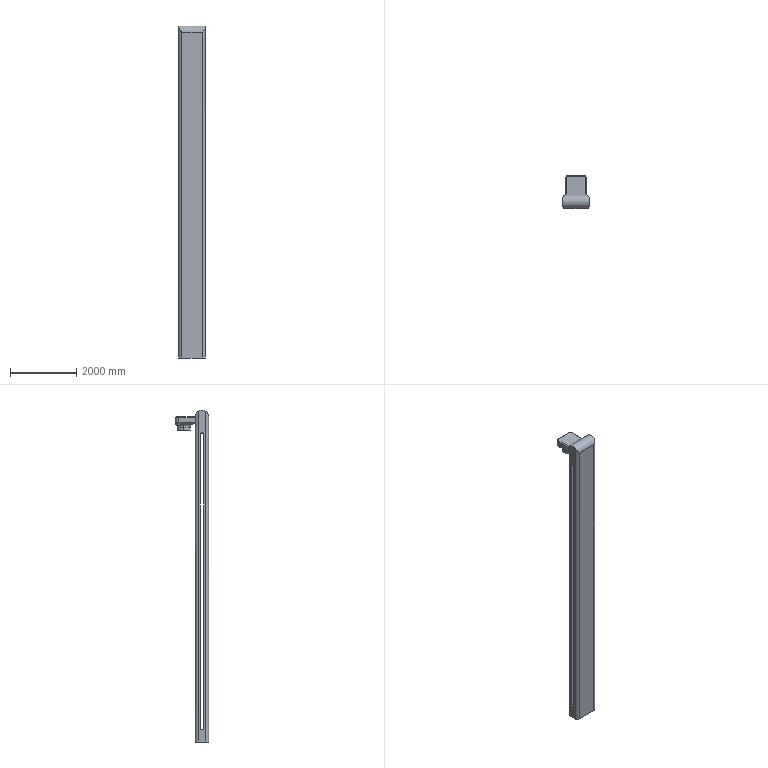Part | SolidWorks | features ICE 9, Fillet 2, Chamfer 1, Extrusion 1 | 1 solid | 53 faces | box 800 x 1000 x 10000 mm | volume 2403832717 mm3 | plane 25 | cylinder 15 | spline 6 | cone 4 | torus 3 | commonest cylinder face diameters 400 x5 180 x4 113.782 x2 200 x2 250 x2